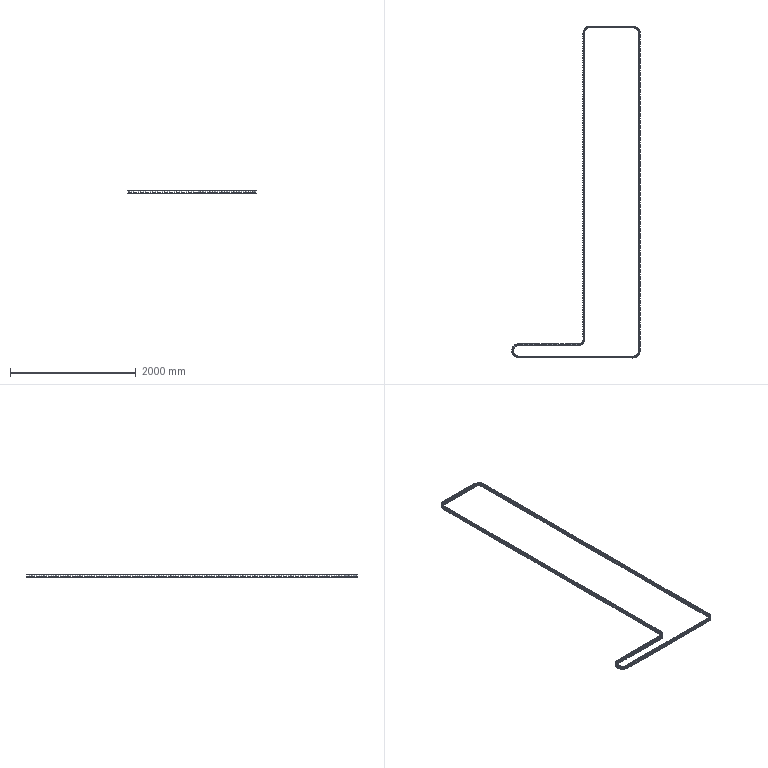Part | STEP file | Outer chain 1-1XG | 187 solids | 5610 faces | volume 4555438 mm3 | cylinder 4114 | plane 1496 | commonest cylinder face diameters 11 x2244 30 x1122 64.25 x748